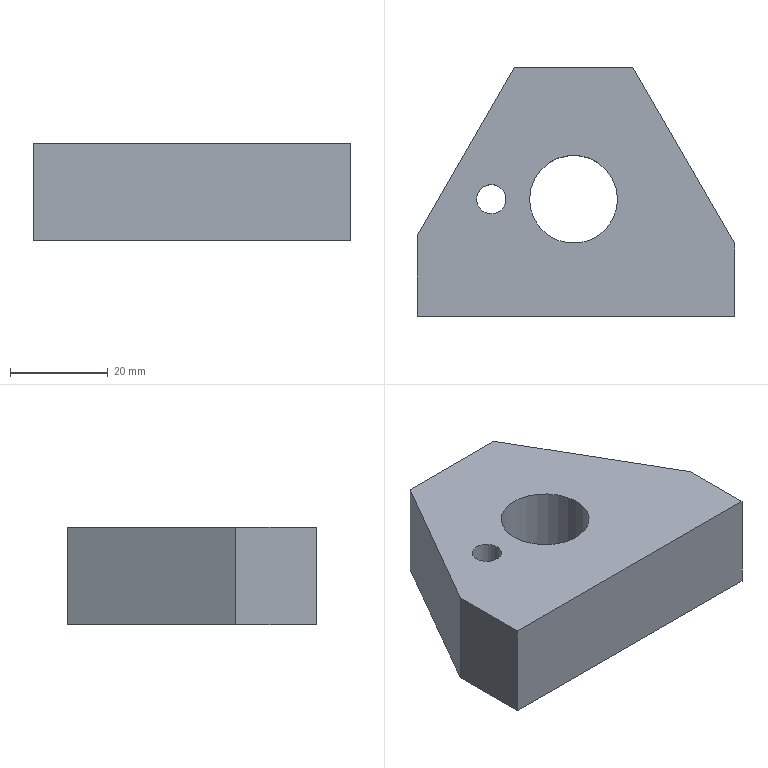Part | NX | 1 solid | 10 faces | box 65 x 51 x 20 mm | volume 46255 mm3 | plane 8 | cylinder 2 | commonest cylinder face diameters 6 x1 18 x1
STEP:
#1=CARTESIAN_POINT('',(-12.124,27.,20.));
#2=VERTEX_POINT('',#1);
#3=CARTESIAN_POINT('',(-12.124,27.,0.));
#4=VERTEX_POINT('',#3);
#5=CARTESIAN_POINT('',(-12.124,27.,20.));
#6=DIRECTION('',(0.,0.,1.));
#7=VECTOR('',#6,1000.);
#8=LINE('',#5,#7);
#9=EDGE_CURVE('',#2,#4,#8,.F.);
#10=ORIENTED_EDGE('',*,*,#9,.T.);
#11=CARTESIAN_POINT('',(-32.,-7.426,0.));
#12=VERTEX_POINT('',#11);
#13=CARTESIAN_POINT('',(0.,48.,0.));
#14=DIRECTION('',(-0.5,-0.866,0.));
#15=VECTOR('',#14,1000.);
#16=LINE('',#13,#15);
#17=EDGE_CURVE('',#4,#12,#16,.T.);
#18=ORIENTED_EDGE('',*,*,#17,.T.);
#19=CARTESIAN_POINT('',(-32.,-7.426,20.));
#20=VERTEX_POINT('',#19);
#21=CARTESIAN_POINT('',(-32.,-7.426,20.));
#22=DIRECTION('',(0.,0.,-1.));
#23=VECTOR('',#22,1000.);
#24=LINE('',#21,#23);
#25=EDGE_CURVE('',#12,#20,#24,.F.);
#26=ORIENTED_EDGE('',*,*,#25,.T.);
#27=CARTESIAN_POINT('',(0.,48.,20.));
#28=DIRECTION('',(-0.5,-0.866,0.));
#29=VECTOR('',#28,1000.);
#30=LINE('',#27,#29);
#31=EDGE_CURVE('',#2,#20,#30,.T.);
#32=ORIENTED_EDGE('',*,*,#31,.F.);
#33=EDGE_LOOP('',(#10,#18,#26,#32));
#34=FACE_BOUND('',#33,.T.);
#35=CARTESIAN_POINT('',(0.,48.,20.));
#36=DIRECTION('',(0.866,-0.5,0.));
#37=DIRECTION('',(0.5,0.866,0.));
#38=AXIS2_PLACEMENT_3D('',#35,#36,#37);
#39=PLANE('',#38);
#40=ADVANCED_FACE('',(#34),#39,.F.);
#41=CARTESIAN_POINT('',(33.,-24.,0.));
#42=VERTEX_POINT('',#41);
#43=CARTESIAN_POINT('',(33.,-24.,20.));
#44=VERTEX_POINT('',#43);
#45=CARTESIAN_POINT('',(33.,-24.,20.));
#46=DIRECTION('',(0.,0.,-1.));
#47=VECTOR('',#46,1000.);
#48=LINE('',#45,#47);
#49=EDGE_CURVE('',#42,#44,#48,.F.);
#50=ORIENTED_EDGE('',*,*,#49,.T.);
#51=CARTESIAN_POINT('',(-32.,-24.,20.));
#52=VERTEX_POINT('',#51);
#53=CARTESIAN_POINT('',(-41.569,-24.,20.));
#54=DIRECTION('',(1.,0.,0.));
#55=VECTOR('',#54,1000.);
#56=LINE('',#53,#55);
#57=EDGE_CURVE('',#52,#44,#56,.T.);
#58=ORIENTED_EDGE('',*,*,#57,.F.);
#59=CARTESIAN_POINT('',(-32.,-24.,0.));
#60=VERTEX_POINT('',#59);
#61=CARTESIAN_POINT('',(-32.,-24.,20.));
#62=DIRECTION('',(0.,0.,1.));
#63=VECTOR('',#62,1000.);
#64=LINE('',#61,#63);
#65=EDGE_CURVE('',#52,#60,#64,.F.);
#66=ORIENTED_EDGE('',*,*,#65,.T.);
#67=CARTESIAN_POINT('',(-41.569,-24.,0.));
#68=DIRECTION('',(1.,0.,0.));
#69=VECTOR('',#68,1000.);
#70=LINE('',#67,#69);
#71=EDGE_CURVE('',#60,#42,#70,.T.);
#72=ORIENTED_EDGE('',*,*,#71,.T.);
#73=EDGE_LOOP('',(#50,#58,#66,#72));
#74=FACE_BOUND('',#73,.T.);
#75=CARTESIAN_POINT('',(-41.569,-24.,20.));
#76=DIRECTION('',(0.,1.,0.));
#77=DIRECTION('',(-1.,0.,0.));
#78=AXIS2_PLACEMENT_3D('',#75,#76,#77);
#79=PLANE('',#78);
#80=ADVANCED_FACE('',(#74),#79,.F.);
#81=CARTESIAN_POINT('',(12.124,27.,0.));
#82=VERTEX_POINT('',#81);
#83=CARTESIAN_POINT('',(12.124,27.,20.));
#84=VERTEX_POINT('',#83);
#85=CARTESIAN_POINT('',(12.124,27.,20.));
#86=DIRECTION('',(0.,0.,-1.));
#87=VECTOR('',#86,1000.);
#88=LINE('',#85,#87);
#89=EDGE_CURVE('',#82,#84,#88,.F.);
#90=ORIENTED_EDGE('',*,*,#89,.T.);
#91=CARTESIAN_POINT('',(33.,-9.158,20.));
#92=VERTEX_POINT('',#91);
#93=CARTESIAN_POINT('',(41.569,-24.,20.));
#94=DIRECTION('',(-0.5,0.866,0.));
#95=VECTOR('',#94,1000.);
#96=LINE('',#93,#95);
#97=EDGE_CURVE('',#92,#84,#96,.T.);
#98=ORIENTED_EDGE('',*,*,#97,.F.);
#99=CARTESIAN_POINT('',(33.,-9.158,0.));
#100=VERTEX_POINT('',#99);
#101=CARTESIAN_POINT('',(33.,-9.158,20.));
#102=DIRECTION('',(0.,0.,1.));
#103=VECTOR('',#102,1000.);
#104=LINE('',#101,#103);
#105=EDGE_CURVE('',#100,#92,#104,.T.);
#106=ORIENTED_EDGE('',*,*,#105,.F.);
#107=CARTESIAN_POINT('',(41.569,-24.,0.));
#108=DIRECTION('',(-0.5,0.866,0.));
#109=VECTOR('',#108,1000.);
#110=LINE('',#107,#109);
#111=EDGE_CURVE('',#100,#82,#110,.T.);
#112=ORIENTED_EDGE('',*,*,#111,.T.);
#113=EDGE_LOOP('',(#90,#98,#106,#112));
#114=FACE_BOUND('',#113,.T.);
#115=CARTESIAN_POINT('',(41.569,-24.,20.));
#116=DIRECTION('',(-0.866,-0.5,0.));
#117=DIRECTION('',(0.5,-0.866,0.));
#118=AXIS2_PLACEMENT_3D('',#115,#116,#117);
#119=PLANE('',#118);
#120=ADVANCED_FACE('',(#114),#119,.F.);
#121=CARTESIAN_POINT('',(9.,0.,0.));
#122=VERTEX_POINT('',#121);
#123=CARTESIAN_POINT('',(0.,0.,0.));
#124=DIRECTION('',(0.,0.,1.));
#125=DIRECTION('',(1.,0.,0.));
#126=AXIS2_PLACEMENT_3D('',#123,#124,#125);
#127=CIRCLE('',#126,9.);
#128=EDGE_CURVE('',#122,#122,#127,.T.);
#129=ORIENTED_EDGE('',*,*,#128,.T.);
#130=EDGE_LOOP('',(#129));
#131=FACE_BOUND('',#130,.T.);
#132=CARTESIAN_POINT('',(-13.85,0.,0.));
#133=VERTEX_POINT('',#132);
#134=CARTESIAN_POINT('',(-16.85,0.,0.));
#135=DIRECTION('',(0.,0.,1.));
#136=DIRECTION('',(1.,0.,0.));
#137=AXIS2_PLACEMENT_3D('',#134,#135,#136);
#138=CIRCLE('',#137,3.);
#139=EDGE_CURVE('',#133,#133,#138,.T.);
#140=ORIENTED_EDGE('',*,*,#139,.T.);
#141=EDGE_LOOP('',(#140));
#142=FACE_BOUND('',#141,.T.);
#143=CARTESIAN_POINT('',(33.,0.,0.));
#144=DIRECTION('',(0.,1.,0.));
#145=VECTOR('',#144,1000.);
#146=LINE('',#143,#145);
#147=EDGE_CURVE('',#42,#100,#146,.T.);
#148=ORIENTED_EDGE('',*,*,#147,.F.);
#149=ORIENTED_EDGE('',*,*,#71,.F.);
#150=CARTESIAN_POINT('',(-32.,0.,0.));
#151=DIRECTION('',(0.,-1.,0.));
#152=VECTOR('',#151,1000.);
#153=LINE('',#150,#152);
#154=EDGE_CURVE('',#12,#60,#153,.T.);
#155=ORIENTED_EDGE('',*,*,#154,.F.);
#156=ORIENTED_EDGE('',*,*,#17,.F.);
#157=CARTESIAN_POINT('',(0.5,27.,0.));
#158=DIRECTION('',(-1.,0.,0.));
#159=VECTOR('',#158,1000.);
#160=LINE('',#157,#159);
#161=EDGE_CURVE('',#82,#4,#160,.T.);
#162=ORIENTED_EDGE('',*,*,#161,.F.);
#163=ORIENTED_EDGE('',*,*,#111,.F.);
#164=EDGE_LOOP('',(#148,#149,#155,#156,#162,#163));
#165=FACE_BOUND('',#164,.T.);
#166=CARTESIAN_POINT('',(-16.85,0.,0.));
#167=DIRECTION('',(0.,0.,1.));
#168=DIRECTION('',(1.,0.,0.));
#169=AXIS2_PLACEMENT_3D('',#166,#167,#168);
#170=PLANE('',#169);
#171=ADVANCED_FACE('',(#131,#142,#165),#170,.F.);
#172=CARTESIAN_POINT('',(-13.85,0.,20.));
#173=VERTEX_POINT('',#172);
#174=CARTESIAN_POINT('',(-16.85,0.,20.));
#175=DIRECTION('',(0.,0.,1.));
#176=DIRECTION('',(1.,0.,0.));
#177=AXIS2_PLACEMENT_3D('',#174,#175,#176);
#178=CIRCLE('',#177,3.);
#179=EDGE_CURVE('',#173,#173,#178,.T.);
#180=ORIENTED_EDGE('',*,*,#179,.T.);
#181=EDGE_LOOP('',(#180));
#182=FACE_BOUND('',#181,.T.);
#183=ORIENTED_EDGE('',*,*,#139,.F.);
#184=EDGE_LOOP('',(#183));
#185=FACE_BOUND('',#184,.T.);
#186=CARTESIAN_POINT('',(-16.85,0.,20.));
#187=DIRECTION('',(0.,0.,-1.));
#188=DIRECTION('',(-1.,0.,0.));
#189=AXIS2_PLACEMENT_3D('',#186,#187,#188);
#190=CYLINDRICAL_SURFACE('',#189,3.);
#191=ADVANCED_FACE('',(#182,#185),#190,.F.);
#192=CARTESIAN_POINT('',(9.,0.,20.));
#193=VERTEX_POINT('',#192);
#194=CARTESIAN_POINT('',(0.,0.,20.));
#195=DIRECTION('',(0.,0.,1.));
#196=DIRECTION('',(1.,0.,0.));
#197=AXIS2_PLACEMENT_3D('',#194,#195,#196);
#198=CIRCLE('',#197,9.);
#199=EDGE_CURVE('',#193,#193,#198,.T.);
#200=ORIENTED_EDGE('',*,*,#199,.T.);
#201=EDGE_LOOP('',(#200));
#202=FACE_BOUND('',#201,.T.);
#203=ORIENTED_EDGE('',*,*,#128,.F.);
#204=EDGE_LOOP('',(#203));
#205=FACE_BOUND('',#204,.T.);
#206=CARTESIAN_POINT('',(0.,0.,20.));
#207=DIRECTION('',(0.,0.,-1.));
#208=DIRECTION('',(-1.,0.,0.));
#209=AXIS2_PLACEMENT_3D('',#206,#207,#208);
#210=CYLINDRICAL_SURFACE('',#209,9.);
#211=ADVANCED_FACE('',(#202,#205),#210,.F.);
#212=CARTESIAN_POINT('',(33.,0.,20.));
#213=DIRECTION('',(0.,-1.,0.));
#214=VECTOR('',#213,1000.);
#215=LINE('',#212,#214);
#216=EDGE_CURVE('',#44,#92,#215,.F.);
#217=ORIENTED_EDGE('',*,*,#216,.T.);
#218=ORIENTED_EDGE('',*,*,#97,.T.);
#219=CARTESIAN_POINT('',(0.5,27.,20.));
#220=DIRECTION('',(1.,0.,0.));
#221=VECTOR('',#220,1000.);
#222=LINE('',#219,#221);
#223=EDGE_CURVE('',#2,#84,#222,.T.);
#224=ORIENTED_EDGE('',*,*,#223,.F.);
#225=ORIENTED_EDGE('',*,*,#31,.T.);
#226=CARTESIAN_POINT('',(-32.,0.,20.));
#227=DIRECTION('',(0.,1.,0.));
#228=VECTOR('',#227,1000.);
#229=LINE('',#226,#228);
#230=EDGE_CURVE('',#20,#52,#229,.F.);
#231=ORIENTED_EDGE('',*,*,#230,.T.);
#232=ORIENTED_EDGE('',*,*,#57,.T.);
#233=EDGE_LOOP('',(#217,#218,#224,#225,#231,#232));
#234=FACE_BOUND('',#233,.T.);
#235=ORIENTED_EDGE('',*,*,#179,.F.);
#236=EDGE_LOOP('',(#235));
#237=FACE_BOUND('',#236,.T.);
#238=ORIENTED_EDGE('',*,*,#199,.F.);
#239=EDGE_LOOP('',(#238));
#240=FACE_BOUND('',#239,.T.);
#241=CARTESIAN_POINT('',(-16.85,0.,20.));
#242=DIRECTION('',(0.,0.,1.));
#243=DIRECTION('',(1.,0.,0.));
#244=AXIS2_PLACEMENT_3D('',#241,#242,#243);
#245=PLANE('',#244);
#246=ADVANCED_FACE('',(#234,#237,#240),#245,.T.);
#247=ORIENTED_EDGE('',*,*,#216,.F.);
#248=ORIENTED_EDGE('',*,*,#49,.F.);
#249=ORIENTED_EDGE('',*,*,#147,.T.);
#250=ORIENTED_EDGE('',*,*,#105,.T.);
#251=EDGE_LOOP('',(#247,#248,#249,#250));
#252=FACE_BOUND('',#251,.T.);
#253=CARTESIAN_POINT('',(33.,0.,0.));
#254=DIRECTION('',(1.,0.,0.));
#255=DIRECTION('',(0.,0.,-1.));
#256=AXIS2_PLACEMENT_3D('',#253,#254,#255);
#257=PLANE('',#256);
#258=ADVANCED_FACE('',(#252),#257,.T.);
#259=ORIENTED_EDGE('',*,*,#161,.T.);
#260=ORIENTED_EDGE('',*,*,#9,.F.);
#261=ORIENTED_EDGE('',*,*,#223,.T.);
#262=ORIENTED_EDGE('',*,*,#89,.F.);
#263=EDGE_LOOP('',(#259,#260,#261,#262));
#264=FACE_BOUND('',#263,.T.);
#265=CARTESIAN_POINT('',(0.5,27.,0.));
#266=DIRECTION('',(0.,1.,0.));
#267=DIRECTION('',(0.,0.,1.));
#268=AXIS2_PLACEMENT_3D('',#265,#266,#267);
#269=PLANE('',#268);
#270=ADVANCED_FACE('',(#264),#269,.T.);
#271=ORIENTED_EDGE('',*,*,#230,.F.);
#272=ORIENTED_EDGE('',*,*,#25,.F.);
#273=ORIENTED_EDGE('',*,*,#154,.T.);
#274=ORIENTED_EDGE('',*,*,#65,.F.);
#275=EDGE_LOOP('',(#271,#272,#273,#274));
#276=FACE_BOUND('',#275,.T.);
#277=CARTESIAN_POINT('',(-32.,0.,0.));
#278=DIRECTION('',(-1.,0.,0.));
#279=DIRECTION('',(0.,0.,1.));
#280=AXIS2_PLACEMENT_3D('',#277,#278,#279);
#281=PLANE('',#280);
#282=ADVANCED_FACE('',(#276),#281,.T.);
#283=CLOSED_SHELL('',(#40,#80,#120,#171,#191,#211,#246,#258,#270,#282));
#284=MANIFOLD_SOLID_BREP('',#283);
#285=(LENGTH_UNIT()NAMED_UNIT(*)SI_UNIT(.MILLI.,.METRE.));
#286=UNCERTAINTY_MEASURE_WITH_UNIT(LENGTH_MEASURE(0.00001),#285,'','');
#287=(NAMED_UNIT(*)PLANE_ANGLE_UNIT()SI_UNIT($,.RADIAN.));
#288=(NAMED_UNIT(*)SI_UNIT($,.STERADIAN.)SOLID_ANGLE_UNIT());
#289=(GEOMETRIC_REPRESENTATION_CONTEXT(3)GLOBAL_UNCERTAINTY_ASSIGNED_CONTEXT((#286))GLOBAL_UNIT_ASSIGNED_CONTEXT((#285,#287,#288))REPRESENTATION_CONTEXT('',''));
#290=ADVANCED_BREP_SHAPE_REPRESENTATION('',(#284),#289);